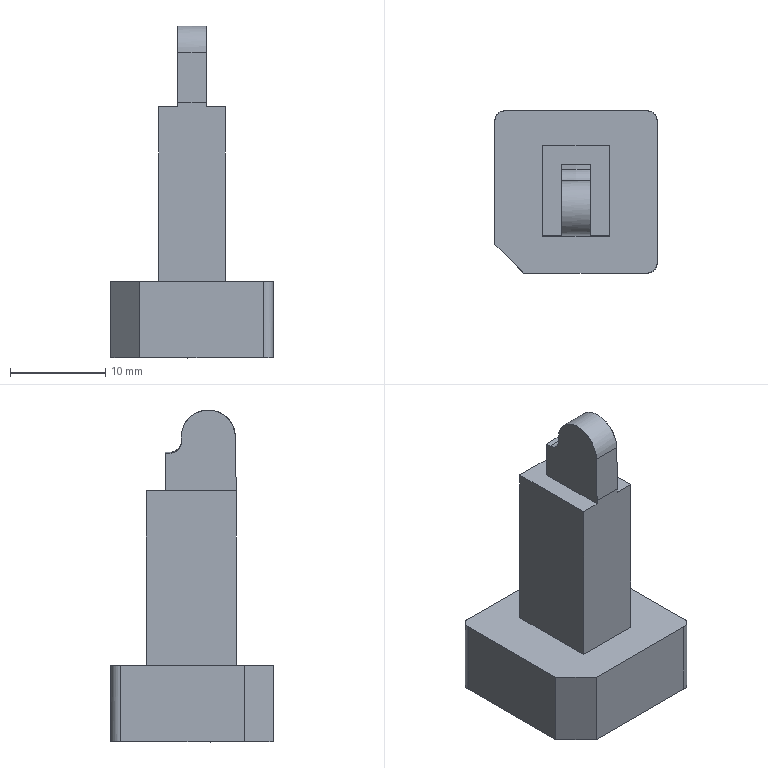CAM job | PowerMill | 3-axis milling, other | part box 17 x 17 x 34.811 mm
Tools:
number,name,type,diameter,tip_radius,length,cutting_length,overhang,flutes,holder,toolpaths_using
1,D10C_1_1_1,end_mill,10.0,0.0,60.0,,35.28,1,D42L35,6
3,D10_1_1_1,end_mill,10.0,0.0,60.0,,34.96,1,D42L35,8
4,R1_1_1,ball_nosed,2.0,1.0,3.0,,4.84,1,D42L35,2
14,D4_1_1,end_mill,4.0,0.0,30.0,,8.76,1,D42L35,1
13,Text_D4_1_1,taper_spherical,4.0,0.3,60.0,,27.08,1,D42L35,2
14,D4_2_1,end_mill,4.0,0.0,30.0,,8.64,1,D42L35,1
Operations:
program,toolpath,strategy,tool,tool_number,tool_diameter,tip_radius,flutes,spindle_rpm,feed_cut,surface_speed_m_min_computed,feed_per_tooth_computed,tolerance,thickness,stepover,stepdown,cut_length,cut_time_min,total_time_min,workplane
04-B01-4-F,精公开粗01-扫面平行-D10C,raster_area_clear,D10C_1_1_1,1,10.0,0.0,1.0,8000.0,10000.0,251.33,1.25,0.03,0.28,6.0,1.0,135.36,0.013,0.0178,
04-B01-4-F,精公开粗01-外形偏置-D10C,offset_area_clear,D10C_1_1_1,1,10.0,0.0,1.0,8000.0,10000.0,251.33,1.25,0.03,0.28,6.0,1.0,10878.907,1.088,1.255,
04-B01-4-F,精公开粗01-基准台等高-D10C,constantz,D10C_1_1_1,1,10.0,0.0,1.0,8000.0,10000.0,251.33,1.25,0.03,0.07,5.0,0.4,2129.058,0.213,0.2252,
04-B01-4-F,精公基准台01-平坦面平行-D10,raster_area_clear,D10_1_1_1,3,10.0,0.0,1.0,8500.0,600.0,267.04,0.0706,0.005,0.38,5.0,1.0,68.326,0.114,0.1486,
04-B01-4-F,精公基准台01-基准面偏置-D10,offset_area_clear,D10_1_1_1,3,10.0,0.0,1.0,8500.0,600.0,267.04,0.0706,0.005,0.38,5.0,1.0,77.201,0.129,0.1502,
04-B01-4-F,精公基准台01-外形侧光-D10,profile_area_clear,D10_1_1_1,3,10.0,0.0,1.0,8500.0,600.0,267.04,0.0706,0.005,-0.07,0.08,1.0,256.59,0.428,0.5449,
04-B01-4-F,精公基准台01-基准台侧光-D10,profile_area_clear,D10_1_1_1,3,10.0,0.0,1.0,8500.0,600.0,267.04,0.0706,0.005,0.0,0.08,1.0,193.234,0.322,0.3889,
04-B01-4-F,精公精光01-平行-R1,raster,R1_1_1,4,2.0,1.0,1.0,18000.0,2000.0,113.1,0.1111,0.005,-0.075,0.03,1.0,1321.35,0.661,0.6734,
04-B01-4-F,精公精光02-等高-D4,constantz,D4_1_1,14,4.0,0.0,1.0,18000.0,2000.0,226.19,0.1111,0.005,-0.075,5.0,0.04,6563.462,3.282,3.292,
04-B01-4-F,精公刻字01-刻字-Text_D4,pattern,Text_D4_1_1,13,4.0,0.3,1.0,15000.0,1000.0,188.5,0.0667,0.005,0.0,5.0,1.0,27.766,0.028,0.0563,
04-B01-4-R,粗公开粗01-扫面平行-D10C,raster_area_clear,D10C_1_1_1,1,10.0,0.0,1.0,8000.0,10000.0,251.33,1.25,0.03,0.15,6.0,1.0,267.6,0.027,0.0329,
04-B01-4-R,粗公开粗01-外形偏置-D10C,offset_area_clear,D10C_1_1_1,1,10.0,0.0,1.0,8000.0,10000.0,251.33,1.25,0.03,0.15,6.0,1.0,10752.295,1.075,1.243,
04-B01-4-R,粗公开粗01-基准台等高-D10C,constantz,D10C_1_1_1,1,10.0,0.0,1.0,8000.0,10000.0,251.33,1.25,0.03,0.07,5.0,0.4,2129.058,0.213,0.2252,
04-B01-4-R,粗公基准台01-平坦面平行-D10,raster_area_clear,D10_1_1_1,3,10.0,0.0,1.0,8500.0,600.0,267.04,0.0706,0.01,0.25,5.0,1.0,96.754,0.161,0.207,
04-B01-4-R,粗公基准台01-基准面偏置-D10,offset_area_clear,D10_1_1_1,3,10.0,0.0,1.0,8500.0,600.0,267.04,0.0706,0.01,0.25,5.0,1.0,76.825,0.128,0.1495,
04-B01-4-R,粗公基准台01-外形侧光-D10,profile_area_clear,D10_1_1_1,3,10.0,0.0,1.0,8500.0,600.0,267.04,0.0706,0.01,-0.2,0.08,1.0,253.323,0.422,0.5395,
04-B01-4-R,粗公基准台01-基准台侧光-D10,profile_area_clear,D10_1_1_1,3,10.0,0.0,1.0,8500.0,600.0,267.04,0.0706,0.01,0.0,0.08,1.0,193.218,0.322,0.3888,
04-B01-4-R,粗公精光01-平行-R1,raster,R1_1_1,4,2.0,1.0,1.0,18000.0,2000.0,113.1,0.1111,0.01,-0.205,0.036,1.0,1059.229,0.53,0.5422,
04-B01-4-R,粗公精光02-等高-D4,constantz,D4_2_1,14,4.0,0.0,1.0,18000.0,2000.0,226.19,0.1111,0.01,-0.205,5.0,0.048,5276.082,2.638,2.647,
04-B01-4-R,粗公刻字01-刻字-Text_D4,pattern,Text_D4_1_1,13,4.0,0.3,1.0,15000.0,1000.0,188.5,0.0667,0.01,0.0,5.0,1.0,27.445,0.027,0.0547,